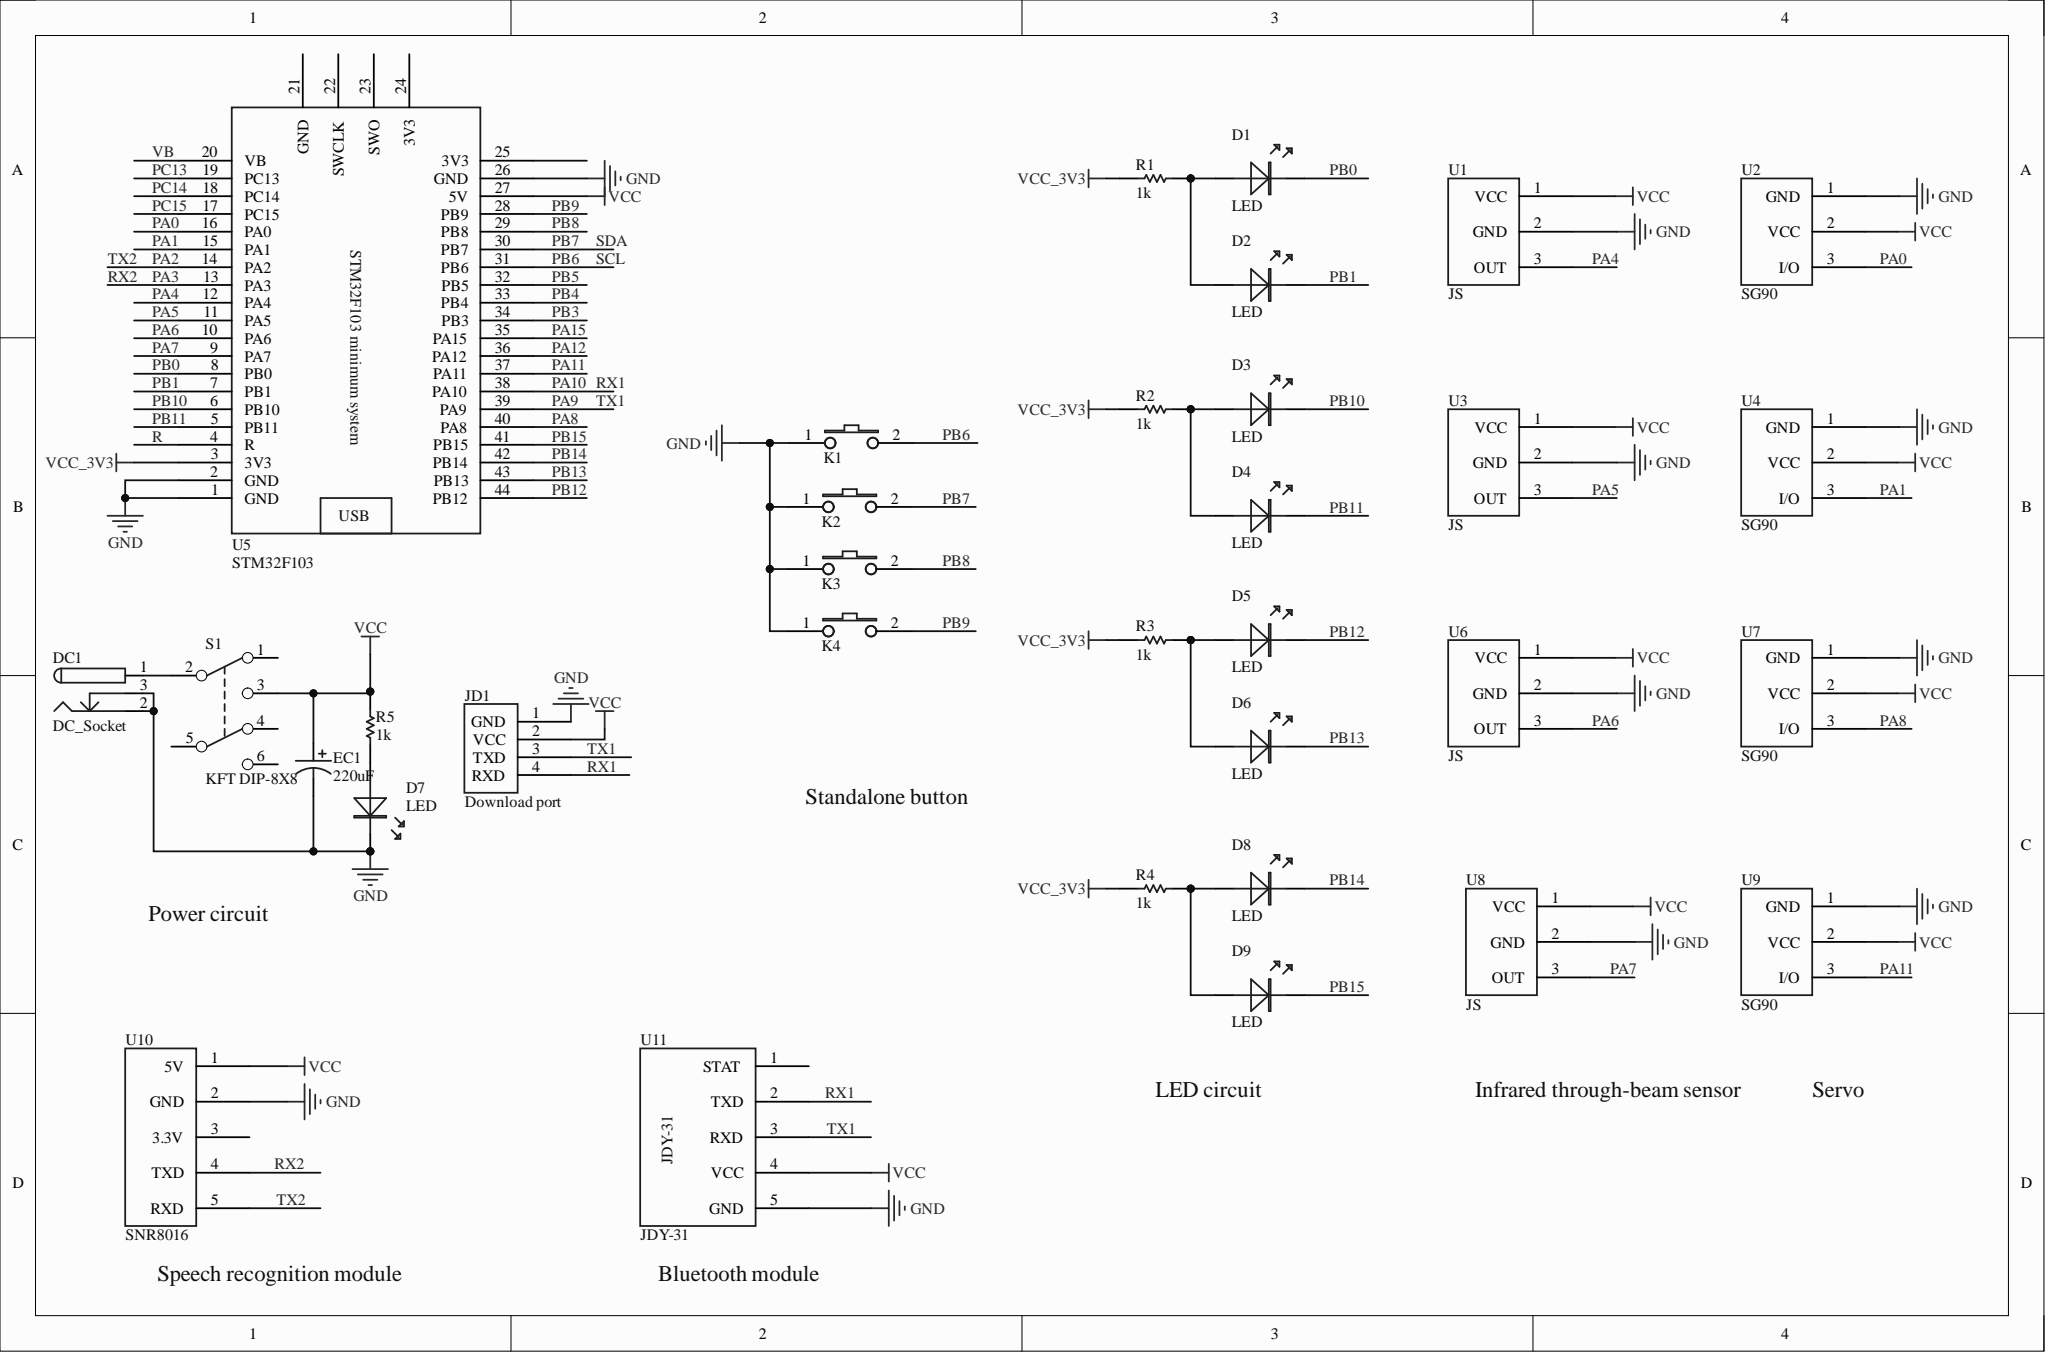Circuit board | Altium Designer | 33 parts | 33 nets
Bill of materials:
Comment,Description,Designator,Footprint,LibRef,Quantity
"LED","Red LED, Green LED","D1, D3, D5, D7, D8","LED5-GRE","LED","5"
"LED","Red LED","D2, D4, D6, D9","LED5-RED","LED_1","4"
"DC_Socket","Power socket","DC1","DC-005","DC_Socket","1"
"220uF","Through-hole electrolytic capacitor","EC1","DIP-EC3.5X8X11.5","220uF","1"
"Download port","Download port","JD1","下载口","下载口_1","1"
"BUTTOM","Button","K1, K2, K3, K4","DIP-6X6X5","BUTTOM","4"
"1k","Resistor","R1, R2, R3, R4, R5","AXIAL0.3-1k","1k","5"
"KFT DIP-8X8","Self-locking button","S1","KFT DIP-8X8","KFT DIP-8X8_1","1"
"JS","Infrared through-beam sensor--counting","U1, U3, U6, U8","JS","JS_2","4"
"SG90","Servo","U2, U4, U7, U9","SG90","SG90_1","4"
"STM32F103","STM32F103","U5","STM32F103","STM32F103_1","1"
"SNR8016","Speech recognition module","U10","SNR8016","SNR8016_1","1"
"JDY-31","Bluetooth","U11","","JDY-31","1"
Netlist (Protel format):
[
D1
LED5-GRE
LED



]
[
D2
LED5-RED
LED



]
[
D3
LED5-GRE
LED



]
[
D4
LED5-RED
LED



]
[
D5
LED5-GRE
LED



]
[
D6
LED5-RED
LED



]
[
D7
LED5-GRE
LED



]
[
D8
LED5-GRE
LED



]
[
D9
LED5-RED
LED



]
[
DC1
DC-005
DC_Socket



]
[
EC1
DIP-EC3.5X8X11.5
220uF



]
[
JD1
下载口
Download port



]
[
K1
DIP-6X6X5
BUTTOM



]
[
K2
DIP-6X6X5
BUTTOM



]
[
K3
DIP-6X6X5
BUTTOM



]
[
K4
DIP-6X6X5
BUTTOM



]
[
R1
AXIAL0.3-1k
1k



]
[
R2
AXIAL0.3-1k
1k



]
[
R3
AXIAL0.3-1k
1k



]
[
R4
AXIAL0.3-1k
1k



]
[
R5
AXIAL0.3-1k
1k



]
[
S1
KFT DIP-8X8
KFT DIP-8X8



]
[
U1
JS
JS



]
[
U2
SG90
SG90



]
[
U3
JS
JS



]
[
U4
SG90
SG90



]
[
U5
STM32F103
STM32F103



]
[
U6
JS
JS



]
[
U7
SG90
SG90



]
[
U8
JS
JS



]
[
U9
SG90
SG90



]
[
U10
SNR8016
SNR8016



]
[
U11

JDY-31



]
(
VCC_3V3
R1-2
R2-2
R3-2
R4-2
U5-3
)
(
VCC
EC1-1
JD1-2
R5-2
S1-3
U1-1
U2-2
U3-1
U4-2
U5-27
U6-1
U7-2
U8-1
U9-2
U10-1
U11-4
)
(
PB15
D9-K
U5-41
)
(
PB14
D8-K
U5-42
)
(
PB13
D6-K
U5-43
)
(
PB12
D5-K
U5-44
)
(
PB11
D4-K
U5-5
)
(
PB10
D3-K
U5-6
)
(
PB9
K4-2
U5-28
)
(
PB8
K3-2
U5-29
)
(
PB7
K2-2
U5-30
)
(
PB6
K1-2
U5-31
)
(
PB1
D2-K
U5-7
)
(
PB0
D1-K
U5-8
)
(
PA11
U5-37
U9-3
)
(
PA10
JD1-4
U5-38
U11-2
)
(
PA9
JD1-3
U5-39
U11-3
)
(
PA8
U5-40
U7-3
)
(
PA7
U5-9
U8-3
)
(
PA6
U5-10
U6-3
)
(
PA5
U3-3
U5-11
)
(
PA4
U1-3
U5-12
)
(
PA3
U5-13
U10-4
)
(
PA2
U5-14
U10-5
)
(
PA1
U4-3
U5-15
)
(
PA0
U2-3
U5-16
)
(
NetDC1_1
DC1-1
S1-2
)
(
NetD8_A
D8-A
D9-A
R4-1
)
(
NetD7_A
D7-A
R5-1
)
(
NetD5_A
D5-A
D6-A
R3-1
)
(
NetD3_A
D3-A
D4-A
R2-1
)
(
NetD1_A
D1-A
D2-A
R1-1
)
(
GND
D7-K
DC1-2
DC1-3
EC1-2
JD1-1
K1-1
K2-1
K3-1
K4-1
U1-2
U2-1
U3-2
U4-1
U5-1
U5-2
U5-26
U6-2
U7-1
U8-2
U9-1
U10-2
U11-5
)